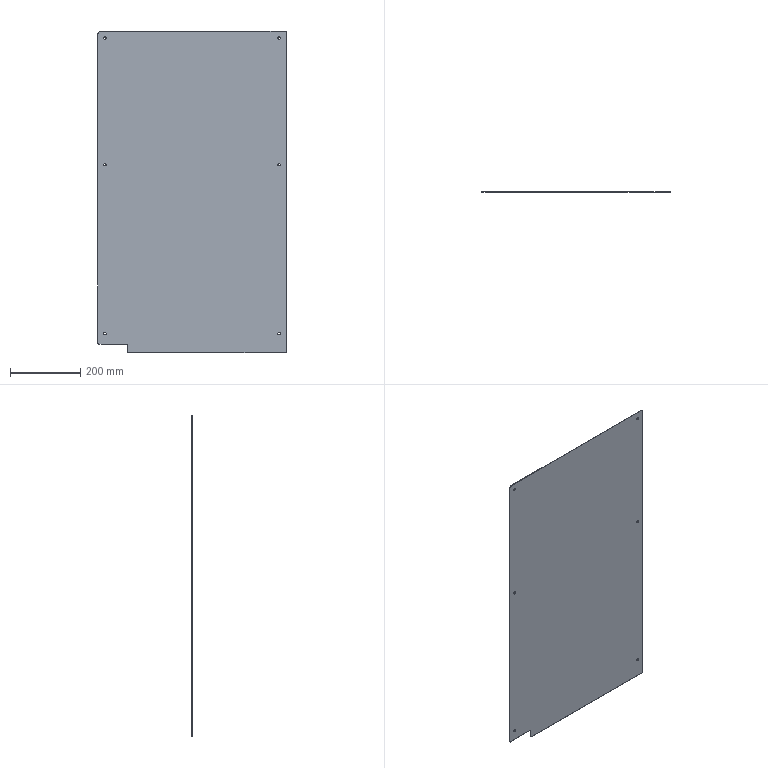Part | SolidWorks | features Fillet 4, ICE 4, FlatPattern 1, HoleWzd 1, SMBaseFlange 1, SheetMetal 1 | 1 solid | 26 faces | box 535 x 1.2 x 915 mm | volume 584570 mm3 | cylinder 18 | plane 8 | commonest cylinder face diameters 7 x12 6 x5 20 x1
STEP:
#1=CARTESIAN_POINT('',(20.,-1.2,-863.5));
#2=VERTEX_POINT('',#1);
#3=CARTESIAN_POINT('',(20.,-1.2,-856.5));
#4=VERTEX_POINT('',#3);
#5=CARTESIAN_POINT('',(20.,-1.2,-860.));
#6=DIRECTION('',(0.,1.,0.));
#7=DIRECTION('',(0.,0.,1.));
#8=AXIS2_PLACEMENT_3D('',#5,#6,#7);
#9=CIRCLE('',#8,3.5);
#10=EDGE_CURVE('',#2,#4,#9,.T.);
#11=ORIENTED_EDGE('',*,*,#10,.F.);
#12=CARTESIAN_POINT('',(20.,0.,-863.5));
#13=VERTEX_POINT('',#12);
#14=CARTESIAN_POINT('',(20.,0.,-863.5));
#15=DIRECTION('',(0.,1.,0.));
#16=VECTOR('',#15,1000.);
#17=LINE('',#14,#16);
#18=EDGE_CURVE('',#2,#13,#17,.T.);
#19=ORIENTED_EDGE('',*,*,#18,.T.);
#20=CARTESIAN_POINT('',(20.,0.,-856.5));
#21=VERTEX_POINT('',#20);
#22=CARTESIAN_POINT('',(20.,0.,-860.));
#23=DIRECTION('',(0.,1.,0.));
#24=DIRECTION('',(0.,0.,1.));
#25=AXIS2_PLACEMENT_3D('',#22,#23,#24);
#26=CIRCLE('',#25,3.5);
#27=EDGE_CURVE('',#13,#21,#26,.T.);
#28=ORIENTED_EDGE('',*,*,#27,.T.);
#29=CARTESIAN_POINT('',(20.,0.,-856.5));
#30=DIRECTION('',(0.,1.,0.));
#31=VECTOR('',#30,1000.);
#32=LINE('',#29,#31);
#33=EDGE_CURVE('',#4,#21,#32,.T.);
#34=ORIENTED_EDGE('',*,*,#33,.F.);
#35=EDGE_LOOP('',(#11,#19,#28,#34));
#36=FACE_OUTER_BOUND('',#35,.T.);
#37=CARTESIAN_POINT('',(20.,0.,-860.));
#38=DIRECTION('',(0.,1.,0.));
#39=DIRECTION('',(0.,0.,1.));
#40=AXIS2_PLACEMENT_3D('',#37,#38,#39);
#41=CYLINDRICAL_SURFACE('',#40,3.5);
#42=ADVANCED_FACE('',(#36),#41,.F.);
#43=CARTESIAN_POINT('',(20.,-1.2,-23.5));
#44=VERTEX_POINT('',#43);
#45=CARTESIAN_POINT('',(20.,-1.2,-16.5));
#46=VERTEX_POINT('',#45);
#47=CARTESIAN_POINT('',(20.,-1.2,-20.));
#48=DIRECTION('',(0.,1.,0.));
#49=DIRECTION('',(0.,0.,1.));
#50=AXIS2_PLACEMENT_3D('',#47,#48,#49);
#51=CIRCLE('',#50,3.5);
#52=EDGE_CURVE('',#44,#46,#51,.T.);
#53=ORIENTED_EDGE('',*,*,#52,.F.);
#54=CARTESIAN_POINT('',(20.,0.,-23.5));
#55=VERTEX_POINT('',#54);
#56=CARTESIAN_POINT('',(20.,0.,-23.5));
#57=DIRECTION('',(0.,1.,0.));
#58=VECTOR('',#57,1000.);
#59=LINE('',#56,#58);
#60=EDGE_CURVE('',#44,#55,#59,.T.);
#61=ORIENTED_EDGE('',*,*,#60,.T.);
#62=CARTESIAN_POINT('',(20.,0.,-16.5));
#63=VERTEX_POINT('',#62);
#64=CARTESIAN_POINT('',(20.,0.,-20.));
#65=DIRECTION('',(0.,1.,0.));
#66=DIRECTION('',(0.,0.,1.));
#67=AXIS2_PLACEMENT_3D('',#64,#65,#66);
#68=CIRCLE('',#67,3.5);
#69=EDGE_CURVE('',#55,#63,#68,.T.);
#70=ORIENTED_EDGE('',*,*,#69,.T.);
#71=CARTESIAN_POINT('',(20.,0.,-16.5));
#72=DIRECTION('',(0.,1.,0.));
#73=VECTOR('',#72,1000.);
#74=LINE('',#71,#73);
#75=EDGE_CURVE('',#46,#63,#74,.T.);
#76=ORIENTED_EDGE('',*,*,#75,.F.);
#77=EDGE_LOOP('',(#53,#61,#70,#76));
#78=FACE_OUTER_BOUND('',#77,.T.);
#79=CARTESIAN_POINT('',(20.,0.,-20.));
#80=DIRECTION('',(0.,1.,0.));
#81=DIRECTION('',(0.,0.,1.));
#82=AXIS2_PLACEMENT_3D('',#79,#80,#81);
#83=CYLINDRICAL_SURFACE('',#82,3.5);
#84=ADVANCED_FACE('',(#78),#83,.F.);
#85=CARTESIAN_POINT('',(515.,-1.2,-23.5));
#86=VERTEX_POINT('',#85);
#87=CARTESIAN_POINT('',(515.,-1.2,-16.5));
#88=VERTEX_POINT('',#87);
#89=CARTESIAN_POINT('',(515.,-1.2,-20.));
#90=DIRECTION('',(0.,1.,0.));
#91=DIRECTION('',(0.,0.,1.));
#92=AXIS2_PLACEMENT_3D('',#89,#90,#91);
#93=CIRCLE('',#92,3.5);
#94=EDGE_CURVE('',#86,#88,#93,.T.);
#95=ORIENTED_EDGE('',*,*,#94,.F.);
#96=CARTESIAN_POINT('',(515.,0.,-23.5));
#97=VERTEX_POINT('',#96);
#98=CARTESIAN_POINT('',(515.,0.,-23.5));
#99=DIRECTION('',(0.,1.,0.));
#100=VECTOR('',#99,1000.);
#101=LINE('',#98,#100);
#102=EDGE_CURVE('',#86,#97,#101,.T.);
#103=ORIENTED_EDGE('',*,*,#102,.T.);
#104=CARTESIAN_POINT('',(515.,0.,-16.5));
#105=VERTEX_POINT('',#104);
#106=CARTESIAN_POINT('',(515.,0.,-20.));
#107=DIRECTION('',(0.,1.,0.));
#108=DIRECTION('',(0.,0.,1.));
#109=AXIS2_PLACEMENT_3D('',#106,#107,#108);
#110=CIRCLE('',#109,3.5);
#111=EDGE_CURVE('',#97,#105,#110,.T.);
#112=ORIENTED_EDGE('',*,*,#111,.T.);
#113=CARTESIAN_POINT('',(515.,0.,-16.5));
#114=DIRECTION('',(0.,1.,0.));
#115=VECTOR('',#114,1000.);
#116=LINE('',#113,#115);
#117=EDGE_CURVE('',#88,#105,#116,.T.);
#118=ORIENTED_EDGE('',*,*,#117,.F.);
#119=EDGE_LOOP('',(#95,#103,#112,#118));
#120=FACE_OUTER_BOUND('',#119,.T.);
#121=CARTESIAN_POINT('',(515.,0.,-20.));
#122=DIRECTION('',(0.,1.,0.));
#123=DIRECTION('',(0.,0.,1.));
#124=AXIS2_PLACEMENT_3D('',#121,#122,#123);
#125=CYLINDRICAL_SURFACE('',#124,3.5);
#126=ADVANCED_FACE('',(#120),#125,.F.);
#127=CARTESIAN_POINT('',(20.,-1.2,-383.5));
#128=VERTEX_POINT('',#127);
#129=CARTESIAN_POINT('',(20.,-1.2,-376.5));
#130=VERTEX_POINT('',#129);
#131=CARTESIAN_POINT('',(20.,-1.2,-380.));
#132=DIRECTION('',(0.,1.,0.));
#133=DIRECTION('',(0.,0.,1.));
#134=AXIS2_PLACEMENT_3D('',#131,#132,#133);
#135=CIRCLE('',#134,3.5);
#136=EDGE_CURVE('',#128,#130,#135,.T.);
#137=ORIENTED_EDGE('',*,*,#136,.F.);
#138=CARTESIAN_POINT('',(20.,0.,-383.5));
#139=VERTEX_POINT('',#138);
#140=CARTESIAN_POINT('',(20.,0.,-383.5));
#141=DIRECTION('',(0.,1.,0.));
#142=VECTOR('',#141,1000.);
#143=LINE('',#140,#142);
#144=EDGE_CURVE('',#128,#139,#143,.T.);
#145=ORIENTED_EDGE('',*,*,#144,.T.);
#146=CARTESIAN_POINT('',(20.,0.,-376.5));
#147=VERTEX_POINT('',#146);
#148=CARTESIAN_POINT('',(20.,0.,-380.));
#149=DIRECTION('',(0.,1.,0.));
#150=DIRECTION('',(0.,0.,1.));
#151=AXIS2_PLACEMENT_3D('',#148,#149,#150);
#152=CIRCLE('',#151,3.5);
#153=EDGE_CURVE('',#139,#147,#152,.T.);
#154=ORIENTED_EDGE('',*,*,#153,.T.);
#155=CARTESIAN_POINT('',(20.,0.,-376.5));
#156=DIRECTION('',(0.,1.,0.));
#157=VECTOR('',#156,1000.);
#158=LINE('',#155,#157);
#159=EDGE_CURVE('',#130,#147,#158,.T.);
#160=ORIENTED_EDGE('',*,*,#159,.F.);
#161=EDGE_LOOP('',(#137,#145,#154,#160));
#162=FACE_OUTER_BOUND('',#161,.T.);
#163=CARTESIAN_POINT('',(20.,0.,-380.));
#164=DIRECTION('',(0.,1.,0.));
#165=DIRECTION('',(0.,0.,1.));
#166=AXIS2_PLACEMENT_3D('',#163,#164,#165);
#167=CYLINDRICAL_SURFACE('',#166,3.5);
#168=ADVANCED_FACE('',(#162),#167,.F.);
#169=CARTESIAN_POINT('',(515.,-1.2,-383.5));
#170=VERTEX_POINT('',#169);
#171=CARTESIAN_POINT('',(515.,-1.2,-376.5));
#172=VERTEX_POINT('',#171);
#173=CARTESIAN_POINT('',(515.,-1.2,-380.));
#174=DIRECTION('',(0.,1.,0.));
#175=DIRECTION('',(0.,0.,1.));
#176=AXIS2_PLACEMENT_3D('',#173,#174,#175);
#177=CIRCLE('',#176,3.5);
#178=EDGE_CURVE('',#170,#172,#177,.T.);
#179=ORIENTED_EDGE('',*,*,#178,.F.);
#180=CARTESIAN_POINT('',(515.,0.,-383.5));
#181=VERTEX_POINT('',#180);
#182=CARTESIAN_POINT('',(515.,0.,-383.5));
#183=DIRECTION('',(0.,1.,0.));
#184=VECTOR('',#183,1000.);
#185=LINE('',#182,#184);
#186=EDGE_CURVE('',#170,#181,#185,.T.);
#187=ORIENTED_EDGE('',*,*,#186,.T.);
#188=CARTESIAN_POINT('',(515.,0.,-376.5));
#189=VERTEX_POINT('',#188);
#190=CARTESIAN_POINT('',(515.,0.,-380.));
#191=DIRECTION('',(0.,1.,0.));
#192=DIRECTION('',(0.,0.,1.));
#193=AXIS2_PLACEMENT_3D('',#190,#191,#192);
#194=CIRCLE('',#193,3.5);
#195=EDGE_CURVE('',#181,#189,#194,.T.);
#196=ORIENTED_EDGE('',*,*,#195,.T.);
#197=CARTESIAN_POINT('',(515.,0.,-376.5));
#198=DIRECTION('',(0.,1.,0.));
#199=VECTOR('',#198,1000.);
#200=LINE('',#197,#199);
#201=EDGE_CURVE('',#172,#189,#200,.T.);
#202=ORIENTED_EDGE('',*,*,#201,.F.);
#203=EDGE_LOOP('',(#179,#187,#196,#202));
#204=FACE_OUTER_BOUND('',#203,.T.);
#205=CARTESIAN_POINT('',(515.,0.,-380.));
#206=DIRECTION('',(0.,1.,0.));
#207=DIRECTION('',(0.,0.,1.));
#208=AXIS2_PLACEMENT_3D('',#205,#206,#207);
#209=CYLINDRICAL_SURFACE('',#208,3.5);
#210=ADVANCED_FACE('',(#204),#209,.F.);
#211=CARTESIAN_POINT('',(515.,-1.2,-863.5));
#212=VERTEX_POINT('',#211);
#213=CARTESIAN_POINT('',(515.,-1.2,-856.5));
#214=VERTEX_POINT('',#213);
#215=CARTESIAN_POINT('',(515.,-1.2,-860.));
#216=DIRECTION('',(0.,1.,0.));
#217=DIRECTION('',(0.,0.,1.));
#218=AXIS2_PLACEMENT_3D('',#215,#216,#217);
#219=CIRCLE('',#218,3.5);
#220=EDGE_CURVE('',#212,#214,#219,.T.);
#221=ORIENTED_EDGE('',*,*,#220,.F.);
#222=CARTESIAN_POINT('',(515.,0.,-863.5));
#223=VERTEX_POINT('',#222);
#224=CARTESIAN_POINT('',(515.,0.,-863.5));
#225=DIRECTION('',(0.,1.,0.));
#226=VECTOR('',#225,1000.);
#227=LINE('',#224,#226);
#228=EDGE_CURVE('',#212,#223,#227,.T.);
#229=ORIENTED_EDGE('',*,*,#228,.T.);
#230=CARTESIAN_POINT('',(515.,0.,-856.5));
#231=VERTEX_POINT('',#230);
#232=CARTESIAN_POINT('',(515.,0.,-860.));
#233=DIRECTION('',(0.,1.,0.));
#234=DIRECTION('',(0.,0.,1.));
#235=AXIS2_PLACEMENT_3D('',#232,#233,#234);
#236=CIRCLE('',#235,3.5);
#237=EDGE_CURVE('',#223,#231,#236,.T.);
#238=ORIENTED_EDGE('',*,*,#237,.T.);
#239=CARTESIAN_POINT('',(515.,0.,-856.5));
#240=DIRECTION('',(0.,1.,0.));
#241=VECTOR('',#240,1000.);
#242=LINE('',#239,#241);
#243=EDGE_CURVE('',#214,#231,#242,.T.);
#244=ORIENTED_EDGE('',*,*,#243,.F.);
#245=EDGE_LOOP('',(#221,#229,#238,#244));
#246=FACE_OUTER_BOUND('',#245,.T.);
#247=CARTESIAN_POINT('',(515.,0.,-860.));
#248=DIRECTION('',(0.,1.,0.));
#249=DIRECTION('',(0.,0.,1.));
#250=AXIS2_PLACEMENT_3D('',#247,#248,#249);
#251=CYLINDRICAL_SURFACE('',#250,3.5);
#252=ADVANCED_FACE('',(#246),#251,.F.);
#253=CARTESIAN_POINT('',(20.,0.,-860.));
#254=DIRECTION('',(0.,1.,0.));
#255=DIRECTION('',(0.,0.,1.));
#256=AXIS2_PLACEMENT_3D('',#253,#254,#255);
#257=CIRCLE('',#256,3.5);
#258=EDGE_CURVE('',#21,#13,#257,.T.);
#259=ORIENTED_EDGE('',*,*,#258,.F.);
#260=ORIENTED_EDGE('',*,*,#27,.F.);
#261=EDGE_LOOP('',(#259,#260));
#262=FACE_BOUND('',#261,.T.);
#263=CARTESIAN_POINT('',(20.,0.,-20.));
#264=DIRECTION('',(0.,1.,0.));
#265=DIRECTION('',(0.,0.,1.));
#266=AXIS2_PLACEMENT_3D('',#263,#264,#265);
#267=CIRCLE('',#266,3.5);
#268=EDGE_CURVE('',#63,#55,#267,.T.);
#269=ORIENTED_EDGE('',*,*,#268,.F.);
#270=ORIENTED_EDGE('',*,*,#69,.F.);
#271=EDGE_LOOP('',(#269,#270));
#272=FACE_BOUND('',#271,.T.);
#273=CARTESIAN_POINT('',(515.,0.,-20.));
#274=DIRECTION('',(0.,1.,0.));
#275=DIRECTION('',(0.,0.,1.));
#276=AXIS2_PLACEMENT_3D('',#273,#274,#275);
#277=CIRCLE('',#276,3.5);
#278=EDGE_CURVE('',#105,#97,#277,.T.);
#279=ORIENTED_EDGE('',*,*,#278,.F.);
#280=ORIENTED_EDGE('',*,*,#111,.F.);
#281=EDGE_LOOP('',(#279,#280));
#282=FACE_BOUND('',#281,.T.);
#283=CARTESIAN_POINT('',(515.,0.,-380.));
#284=DIRECTION('',(0.,1.,0.));
#285=DIRECTION('',(0.,0.,1.));
#286=AXIS2_PLACEMENT_3D('',#283,#284,#285);
#287=CIRCLE('',#286,3.5);
#288=EDGE_CURVE('',#189,#181,#287,.T.);
#289=ORIENTED_EDGE('',*,*,#288,.F.);
#290=ORIENTED_EDGE('',*,*,#195,.F.);
#291=EDGE_LOOP('',(#289,#290));
#292=FACE_BOUND('',#291,.T.);
#293=CARTESIAN_POINT('',(515.,0.,-860.));
#294=DIRECTION('',(0.,1.,0.));
#295=DIRECTION('',(0.,0.,1.));
#296=AXIS2_PLACEMENT_3D('',#293,#294,#295);
#297=CIRCLE('',#296,3.5);
#298=EDGE_CURVE('',#231,#223,#297,.T.);
#299=ORIENTED_EDGE('',*,*,#298,.F.);
#300=ORIENTED_EDGE('',*,*,#237,.F.);
#301=EDGE_LOOP('',(#299,#300));
#302=FACE_BOUND('',#301,.T.);
#303=CARTESIAN_POINT('',(535.,0.,-912.));
#304=VERTEX_POINT('',#303);
#305=CARTESIAN_POINT('',(535.,0.,-3.));
#306=VERTEX_POINT('',#305);
#307=CARTESIAN_POINT('',(535.,0.,-915.));
#308=DIRECTION('',(0.,0.,1.));
#309=VECTOR('',#308,1000.);
#310=LINE('',#307,#309);
#311=EDGE_CURVE('',#304,#306,#310,.T.);
#312=ORIENTED_EDGE('',*,*,#311,.F.);
#313=CARTESIAN_POINT('',(532.,0.,-915.));
#314=VERTEX_POINT('',#313);
#315=CARTESIAN_POINT('',(532.,0.,-912.));
#316=DIRECTION('',(0.,1.,0.));
#317=DIRECTION('',(0.,0.,-1.));
#318=AXIS2_PLACEMENT_3D('',#315,#316,#317);
#319=CIRCLE('',#318,3.);
#320=EDGE_CURVE('',#304,#314,#319,.T.);
#321=ORIENTED_EDGE('',*,*,#320,.T.);
#322=CARTESIAN_POINT('',(88.,0.,-915.));
#323=VERTEX_POINT('',#322);
#324=CARTESIAN_POINT('',(0.,0.,-915.));
#325=DIRECTION('',(-1.,0.,0.));
#326=VECTOR('',#325,1000.);
#327=LINE('',#324,#326);
#328=EDGE_CURVE('',#314,#323,#327,.T.);
#329=ORIENTED_EDGE('',*,*,#328,.T.);
#330=CARTESIAN_POINT('',(85.,0.,-912.));
#331=VERTEX_POINT('',#330);
#332=CARTESIAN_POINT('',(88.,0.,-912.));
#333=DIRECTION('',(0.,1.,0.));
#334=DIRECTION('',(0.,0.,-1.));
#335=AXIS2_PLACEMENT_3D('',#332,#333,#334);
#336=CIRCLE('',#335,3.);
#337=EDGE_CURVE('',#323,#331,#336,.T.);
#338=ORIENTED_EDGE('',*,*,#337,.T.);
#339=CARTESIAN_POINT('',(85.,0.,-893.));
#340=VERTEX_POINT('',#339);
#341=CARTESIAN_POINT('',(85.,0.,-915.));
#342=DIRECTION('',(0.,0.,-1.));
#343=VECTOR('',#342,1000.);
#344=LINE('',#341,#343);
#345=EDGE_CURVE('',#340,#331,#344,.T.);
#346=ORIENTED_EDGE('',*,*,#345,.F.);
#347=CARTESIAN_POINT('',(82.,0.,-890.));
#348=VERTEX_POINT('',#347);
#349=CARTESIAN_POINT('',(82.,0.,-893.));
#350=DIRECTION('',(0.,-1.,0.));
#351=DIRECTION('',(0.,0.,-1.));
#352=AXIS2_PLACEMENT_3D('',#349,#350,#351);
#353=CIRCLE('',#352,3.);
#354=EDGE_CURVE('',#340,#348,#353,.T.);
#355=ORIENTED_EDGE('',*,*,#354,.T.);
#356=CARTESIAN_POINT('',(3.,0.,-890.));
#357=VERTEX_POINT('',#356);
#358=CARTESIAN_POINT('',(0.,0.,-890.));
#359=DIRECTION('',(1.,0.,0.));
#360=VECTOR('',#359,1000.);
#361=LINE('',#358,#360);
#362=EDGE_CURVE('',#357,#348,#361,.T.);
#363=ORIENTED_EDGE('',*,*,#362,.F.);
#364=CARTESIAN_POINT('',(0.,0.,-887.));
#365=VERTEX_POINT('',#364);
#366=CARTESIAN_POINT('',(3.,0.,-887.));
#367=DIRECTION('',(0.,1.,0.));
#368=DIRECTION('',(0.,0.,-1.));
#369=AXIS2_PLACEMENT_3D('',#366,#367,#368);
#370=CIRCLE('',#369,3.);
#371=EDGE_CURVE('',#357,#365,#370,.T.);
#372=ORIENTED_EDGE('',*,*,#371,.T.);
#373=CARTESIAN_POINT('',(0.,0.,-10.));
#374=VERTEX_POINT('',#373);
#375=CARTESIAN_POINT('',(0.,0.,0.));
#376=DIRECTION('',(0.,0.,1.));
#377=VECTOR('',#376,1000.);
#378=LINE('',#375,#377);
#379=EDGE_CURVE('',#365,#374,#378,.T.);
#380=ORIENTED_EDGE('',*,*,#379,.T.);
#381=CARTESIAN_POINT('',(10.,0.,0.));
#382=VERTEX_POINT('',#381);
#383=CARTESIAN_POINT('',(10.,0.,-10.));
#384=DIRECTION('',(0.,1.,0.));
#385=DIRECTION('',(0.,0.,-1.));
#386=AXIS2_PLACEMENT_3D('',#383,#384,#385);
#387=CIRCLE('',#386,10.);
#388=EDGE_CURVE('',#374,#382,#387,.T.);
#389=ORIENTED_EDGE('',*,*,#388,.T.);
#390=CARTESIAN_POINT('',(532.,0.,0.));
#391=VERTEX_POINT('',#390);
#392=CARTESIAN_POINT('',(0.,0.,0.));
#393=DIRECTION('',(1.,0.,0.));
#394=VECTOR('',#393,1000.);
#395=LINE('',#392,#394);
#396=EDGE_CURVE('',#382,#391,#395,.T.);
#397=ORIENTED_EDGE('',*,*,#396,.T.);
#398=CARTESIAN_POINT('',(532.,0.,-3.));
#399=DIRECTION('',(0.,1.,0.));
#400=DIRECTION('',(0.,0.,-1.));
#401=AXIS2_PLACEMENT_3D('',#398,#399,#400);
#402=CIRCLE('',#401,3.);
#403=EDGE_CURVE('',#391,#306,#402,.T.);
#404=ORIENTED_EDGE('',*,*,#403,.T.);
#405=EDGE_LOOP('',(#312,#321,#329,#338,#346,#355,#363,#372,#380,#389,#397,#404));
#406=FACE_OUTER_BOUND('',#405,.T.);
#407=CARTESIAN_POINT('',(20.,0.,-380.));
#408=DIRECTION('',(0.,1.,0.));
#409=DIRECTION('',(0.,0.,1.));
#410=AXIS2_PLACEMENT_3D('',#407,#408,#409);
#411=CIRCLE('',#410,3.5);
#412=EDGE_CURVE('',#147,#139,#411,.T.);
#413=ORIENTED_EDGE('',*,*,#412,.F.);
#414=ORIENTED_EDGE('',*,*,#153,.F.);
#415=EDGE_LOOP('',(#413,#414));
#416=FACE_BOUND('',#415,.T.);
#417=CARTESIAN_POINT('',(0.,0.,0.));
#418=DIRECTION('',(0.,-1.,0.));
#419=DIRECTION('',(0.,0.,-1.));
#420=AXIS2_PLACEMENT_3D('',#417,#418,#419);
#421=PLANE('',#420);
#422=ADVANCED_FACE('',(#262,#272,#282,#292,#302,#406,#416),#421,.F.);
#423=ORIENTED_EDGE('',*,*,#328,.F.);
#424=CARTESIAN_POINT('',(532.,-1.2,-915.));
#425=VERTEX_POINT('',#424);
#426=CARTESIAN_POINT('',(532.,-1.2,-915.));
#427=DIRECTION('',(0.,-1.,0.));
#428=VECTOR('',#427,1000.);
#429=LINE('',#426,#428);
#430=EDGE_CURVE('',#314,#425,#429,.T.);
#431=ORIENTED_EDGE('',*,*,#430,.T.);
#432=CARTESIAN_POINT('',(88.,-1.2,-915.));
#433=VERTEX_POINT('',#432);
#434=CARTESIAN_POINT('',(0.,-1.2,-915.));
#435=DIRECTION('',(-1.,0.,0.));
#436=VECTOR('',#435,1000.);
#437=LINE('',#434,#436);
#438=EDGE_CURVE('',#425,#433,#437,.T.);
#439=ORIENTED_EDGE('',*,*,#438,.T.);
#440=CARTESIAN_POINT('',(88.,0.,-915.));
#441=DIRECTION('',(0.,1.,0.));
#442=VECTOR('',#441,1000.);
#443=LINE('',#440,#442);
#444=EDGE_CURVE('',#433,#323,#443,.T.);
#445=ORIENTED_EDGE('',*,*,#444,.T.);
#446=EDGE_LOOP('',(#423,#431,#439,#445));
#447=FACE_OUTER_BOUND('',#446,.T.);
#448=CARTESIAN_POINT('',(0.,-1.2,-915.));
#449=DIRECTION('',(0.,0.,-1.));
#450=DIRECTION('',(-1.,0.,0.));
#451=AXIS2_PLACEMENT_3D('',#448,#449,#450);
#452=PLANE('',#451);
#453=ADVANCED_FACE('',(#447),#452,.T.);
#454=CARTESIAN_POINT('',(10.,-1.2,0.));
#455=VERTEX_POINT('',#454);
#456=CARTESIAN_POINT('',(532.,-1.2,0.));
#457=VERTEX_POINT('',#456);
#458=CARTESIAN_POINT('',(0.,-1.2,0.));
#459=DIRECTION('',(1.,0.,0.));
#460=VECTOR('',#459,1000.);
#461=LINE('',#458,#460);
#462=EDGE_CURVE('',#455,#457,#461,.T.);
#463=ORIENTED_EDGE('',*,*,#462,.T.);
#464=CARTESIAN_POINT('',(532.,0.,0.));
#465=DIRECTION('',(0.,1.,0.));
#466=VECTOR('',#465,1000.);
#467=LINE('',#464,#466);
#468=EDGE_CURVE('',#457,#391,#467,.T.);
#469=ORIENTED_EDGE('',*,*,#468,.T.);
#470=ORIENTED_EDGE('',*,*,#396,.F.);
#471=CARTESIAN_POINT('',(10.,-1.2,0.));
#472=DIRECTION('',(0.,-1.,0.));
#473=VECTOR('',#472,1000.);
#474=LINE('',#471,#473);
#475=EDGE_CURVE('',#382,#455,#474,.T.);
#476=ORIENTED_EDGE('',*,*,#475,.T.);
#477=EDGE_LOOP('',(#463,#469,#470,#476));
#478=FACE_OUTER_BOUND('',#477,.T.);
#479=CARTESIAN_POINT('',(0.,-1.2,0.));
#480=DIRECTION('',(0.,0.,1.));
#481=DIRECTION('',(1.,0.,0.));
#482=AXIS2_PLACEMENT_3D('',#479,#480,#481);
#483=PLANE('',#482);
#484=ADVANCED_FACE('',(#478),#483,.T.);
#485=CARTESIAN_POINT('',(20.,-1.2,-860.));
#486=DIRECTION('',(0.,1.,0.));
#487=DIRECTION('',(0.,0.,1.));
#488=AXIS2_PLACEMENT_3D('',#485,#486,#487);
#489=CIRCLE('',#488,3.5);
#490=EDGE_CURVE('',#4,#2,#489,.T.);
#491=ORIENTED_EDGE('',*,*,#490,.T.);
#492=ORIENTED_EDGE('',*,*,#10,.T.);
#493=EDGE_LOOP('',(#491,#492));
#494=FACE_BOUND('',#493,.T.);
#495=CARTESIAN_POINT('',(20.,-1.2,-20.));
#496=DIRECTION('',(0.,1.,0.));
#497=DIRECTION('',(0.,0.,1.));
#498=AXIS2_PLACEMENT_3D('',#495,#496,#497);
#499=CIRCLE('',#498,3.5);
#500=EDGE_CURVE('',#46,#44,#499,.T.);
#501=ORIENTED_EDGE('',*,*,#500,.T.);
#502=ORIENTED_EDGE('',*,*,#52,.T.);
#503=EDGE_LOOP('',(#501,#502));
#504=FACE_BOUND('',#503,.T.);
#505=CARTESIAN_POINT('',(515.,-1.2,-20.));
#506=DIRECTION('',(0.,1.,0.));
#507=DIRECTION('',(0.,0.,1.));
#508=AXIS2_PLACEMENT_3D('',#505,#506,#507);
#509=CIRCLE('',#508,3.5);
#510=EDGE_CURVE('',#88,#86,#509,.T.);
#511=ORIENTED_EDGE('',*,*,#510,.T.);
#512=ORIENTED_EDGE('',*,*,#94,.T.);
#513=EDGE_LOOP('',(#511,#512));
#514=FACE_BOUND('',#513,.T.);
#515=CARTESIAN_POINT('',(20.,-1.2,-380.));
#516=DIRECTION('',(0.,1.,0.));
#517=DIRECTION('',(0.,0.,1.));
#518=AXIS2_PLACEMENT_3D('',#515,#516,#517);
#519=CIRCLE('',#518,3.5);
#520=EDGE_CURVE('',#130,#128,#519,.T.);
#521=ORIENTED_EDGE('',*,*,#520,.T.);
#522=ORIENTED_EDGE('',*,*,#136,.T.);
#523=EDGE_LOOP('',(#521,#522));
#524=FACE_BOUND('',#523,.T.);
#525=CARTESIAN_POINT('',(515.,-1.2,-380.));
#526=DIRECTION('',(0.,1.,0.));
#527=DIRECTION('',(0.,0.,1.));
#528=AXIS2_PLACEMENT_3D('',#525,#526,#527);
#529=CIRCLE('',#528,3.5);
#530=EDGE_CURVE('',#172,#170,#529,.T.);
#531=ORIENTED_EDGE('',*,*,#530,.T.);
#532=ORIENTED_EDGE('',*,*,#178,.T.);
#533=EDGE_LOOP('',(#531,#532));
#534=FACE_BOUND('',#533,.T.);
#535=CARTESIAN_POINT('',(515.,-1.2,-860.));
#536=DIRECTION('',(0.,1.,0.));
#537=DIRECTION('',(0.,0.,1.));
#538=AXIS2_PLACEMENT_3D('',#535,#536,#537);
#539=CIRCLE('',#538,3.5);
#540=EDGE_CURVE('',#214,#212,#539,.T.);
#541=ORIENTED_EDGE('',*,*,#540,.T.);
#542=ORIENTED_EDGE('',*,*,#220,.T.);
#543=EDGE_LOOP('',(#541,#542));
#544=FACE_BOUND('',#543,.T.);
#545=ORIENTED_EDGE('',*,*,#438,.F.);
#546=CARTESIAN_POINT('',(535.,-1.2,-912.));
#547=VERTEX_POINT('',#546);
#548=CARTESIAN_POINT('',(532.,-1.2,-912.));
#549=DIRECTION('',(0.,-1.,0.));
#550=DIRECTION('',(0.,0.,-1.));
#551=AXIS2_PLACEMENT_3D('',#548,#549,#550);
#552=CIRCLE('',#551,3.);
#553=EDGE_CURVE('',#425,#547,#552,.T.);
#554=ORIENTED_EDGE('',*,*,#553,.T.);
#555=CARTESIAN_POINT('',(535.,-1.2,-3.));
#556=VERTEX_POINT('',#555);
#557=CARTESIAN_POINT('',(535.,-1.2,0.));
#558=DIRECTION('',(0.,0.,-1.));
#559=VECTOR('',#558,1000.);
#560=LINE('',#557,#559);
#561=EDGE_CURVE('',#556,#547,#560,.T.);
#562=ORIENTED_EDGE('',*,*,#561,.F.);
#563=CARTESIAN_POINT('',(532.,-1.2,-3.));
#564=DIRECTION('',(0.,-1.,0.));
#565=DIRECTION('',(0.,0.,-1.));
#566=AXIS2_PLACEMENT_3D('',#563,#564,#565);
#567=CIRCLE('',#566,3.);
#568=EDGE_CURVE('',#556,#457,#567,.T.);
#569=ORIENTED_EDGE('',*,*,#568,.T.);
#570=ORIENTED_EDGE('',*,*,#462,.F.);
#571=CARTESIAN_POINT('',(0.,-1.2,-10.));
#572=VERTEX_POINT('',#571);
#573=CARTESIAN_POINT('',(10.,-1.2,-10.));
#574=DIRECTION('',(0.,-1.,0.));
#575=DIRECTION('',(0.,0.,-1.));
#576=AXIS2_PLACEMENT_3D('',#573,#574,#575);
#577=CIRCLE('',#576,10.);
#578=EDGE_CURVE('',#455,#572,#577,.T.);
#579=ORIENTED_EDGE('',*,*,#578,.T.);
#580=CARTESIAN_POINT('',(0.,-1.2,-887.));
#581=VERTEX_POINT('',#580);
#582=CARTESIAN_POINT('',(0.,-1.2,0.));
#583=DIRECTION('',(0.,0.,1.));
#584=VECTOR('',#583,1000.);
#585=LINE('',#582,#584);
#586=EDGE_CURVE('',#581,#572,#585,.T.);
#587=ORIENTED_EDGE('',*,*,#586,.F.);
#588=CARTESIAN_POINT('',(3.,-1.2,-890.));
#589=VERTEX_POINT('',#588);
#590=CARTESIAN_POINT('',(3.,-1.2,-887.));
#591=DIRECTION('',(0.,-1.,0.));
#592=DIRECTION('',(0.,0.,-1.));
#593=AXIS2_PLACEMENT_3D('',#590,#591,#592);
#594=CIRCLE('',#593,3.);
#595=EDGE_CURVE('',#581,#589,#594,.T.);
#596=ORIENTED_EDGE('',*,*,#595,.T.);
#597=CARTESIAN_POINT('',(82.,-1.2,-890.));
#598=VERTEX_POINT('',#597);
#599=CARTESIAN_POINT('',(0.,-1.2,-890.));
#600=DIRECTION('',(-1.,0.,0.));
#601=VECTOR('',#600,1000.);
#602=LINE('',#599,#601);
#603=EDGE_CURVE('',#598,#589,#602,.T.);
#604=ORIENTED_EDGE('',*,*,#603,.F.);
#605=CARTESIAN_POINT('',(85.,-1.2,-893.));
#606=VERTEX_POINT('',#605);
#607=CARTESIAN_POINT('',(82.,-1.2,-893.));
#608=DIRECTION('',(0.,1.,0.));
#609=DIRECTION('',(0.,0.,-1.));
#610=AXIS2_PLACEMENT_3D('',#607,#608,#609);
#611=CIRCLE('',#610,3.);
#612=EDGE_CURVE('',#598,#606,#611,.T.);
#613=ORIENTED_EDGE('',*,*,#612,.T.);
#614=CARTESIAN_POINT('',(85.,-1.2,-912.));
#615=VERTEX_POINT('',#614);
#616=CARTESIAN_POINT('',(85.,-1.2,0.));
#617=DIRECTION('',(0.,0.,1.));
#618=VECTOR('',#617,1000.);
#619=LINE('',#616,#618);
#620=EDGE_CURVE('',#615,#606,#619,.T.);
#621=ORIENTED_EDGE('',*,*,#620,.F.);
#622=CARTESIAN_POINT('',(88.,-1.2,-912.));
#623=DIRECTION('',(0.,-1.,0.));
#624=DIRECTION('',(0.,0.,-1.));
#625=AXIS2_PLACEMENT_3D('',#622,#623,#624);
#626=CIRCLE('',#625,3.);
#627=EDGE_CURVE('',#615,#433,#626,.T.);
#628=ORIENTED_EDGE('',*,*,#627,.T.);
#629=EDGE_LOOP('',(#545,#554,#562,#569,#570,#579,#587,#596,#604,#613,#621,#628));
#630=FACE_OUTER_BOUND('',#629,.T.);
#631=CARTESIAN_POINT('',(0.,-1.2,0.));
#632=DIRECTION('',(0.,-1.,0.));
#633=DIRECTION('',(0.,0.,-1.));
#634=AXIS2_PLACEMENT_3D('',#631,#632,#633);
#635=PLANE('',#634);
#636=ADVANCED_FACE('',(#494,#504,#514,#524,#534,#544,#630),#635,.T.);
#637=ORIENTED_EDGE('',*,*,#379,.F.);
#638=CARTESIAN_POINT('',(0.,-1.2,-887.));
#639=DIRECTION('',(0.,-1.,0.));
#640=VECTOR('',#639,1000.);
#641=LINE('',#638,#640);
#642=EDGE_CURVE('',#365,#581,#641,.T.);
#643=ORIENTED_EDGE('',*,*,#642,.T.);
#644=ORIENTED_EDGE('',*,*,#586,.T.);
#645=CARTESIAN_POINT('',(0.,-1.2,-10.));
#646=DIRECTION('',(0.,1.,0.));
#647=VECTOR('',#646,1000.);
#648=LINE('',#645,#647);
#649=EDGE_CURVE('',#572,#374,#648,.T.);
#650=ORIENTED_EDGE('',*,*,#649,.T.);
#651=EDGE_LOOP('',(#637,#643,#644,#650));
#652=FACE_OUTER_BOUND('',#651,.T.);
#653=CARTESIAN_POINT('',(0.,-1.2,0.));
#654=DIRECTION('',(-1.,0.,0.));
#655=DIRECTION('',(0.,0.,1.));
#656=AXIS2_PLACEMENT_3D('',#653,#654,#655);
#657=PLANE('',#656);
#658=ADVANCED_FACE('',(#652),#657,.T.);
#659=ORIENTED_EDGE('',*,*,#561,.T.);
#660=CARTESIAN_POINT('',(535.,0.,-912.));
#661=DIRECTION('',(0.,1.,0.));
#662=VECTOR('',#661,1000.);
#663=LINE('',#660,#662);
#664=EDGE_CURVE('',#547,#304,#663,.T.);
#665=ORIENTED_EDGE('',*,*,#664,.T.);
#666=ORIENTED_EDGE('',*,*,#311,.T.);
#667=CARTESIAN_POINT('',(535.,-1.2,-3.));
#668=DIRECTION('',(0.,-1.,0.));
#669=VECTOR('',#668,1000.);
#670=LINE('',#667,#669);
#671=EDGE_CURVE('',#306,#556,#670,.T.);
#672=ORIENTED_EDGE('',*,*,#671,.T.);
#673=EDGE_LOOP('',(#659,#665,#666,#672));
#674=FACE_OUTER_BOUND('',#673,.T.);
#675=CARTESIAN_POINT('',(535.,-10.,-915.));
#676=DIRECTION('',(-1.,0.,0.));
#677=DIRECTION('',(0.,0.,1.));
#678=AXIS2_PLACEMENT_3D('',#675,#676,#677);
#679=PLANE('',#678);
#680=ADVANCED_FACE('',(#674),#679,.F.);
#681=ORIENTED_EDGE('',*,*,#345,.T.);
#682=CARTESIAN_POINT('',(85.,-1.2,-912.));
#683=DIRECTION('',(0.,-1.,0.));
#684=VECTOR('',#683,1000.);
#685=LINE('',#682,#684);
#686=EDGE_CURVE('',#331,#615,#685,.T.);
#687=ORIENTED_EDGE('',*,*,#686,.T.);
#688=ORIENTED_EDGE('',*,*,#620,.T.);
#689=CARTESIAN_POINT('',(85.,0.,-893.));
#690=DIRECTION('',(0.,1.,0.));
#691=VECTOR('',#690,1000.);
#692=LINE('',#689,#691);
#693=EDGE_CURVE('',#606,#340,#692,.T.);
#694=ORIENTED_EDGE('',*,*,#693,.T.);
#695=EDGE_LOOP('',(#681,#687,#688,#694));
#696=FACE_OUTER_BOUND('',#695,.T.);
#697=CARTESIAN_POINT('',(85.,-10.,-915.));
#698=DIRECTION('',(1.,0.,0.));
#699=DIRECTION('',(0.,0.,-1.));
#700=AXIS2_PLACEMENT_3D('',#697,#698,#699);
#701=PLANE('',#700);
#702=ADVANCED_FACE('',(#696),#701,.F.);
#703=ORIENTED_EDGE('',*,*,#362,.T.);
#704=CARTESIAN_POINT('',(82.,-1.2,-890.));
#705=DIRECTION('',(0.,-1.,0.));
#706=VECTOR('',#705,1000.);
#707=LINE('',#704,#706);
#708=EDGE_CURVE('',#348,#598,#707,.T.);
#709=ORIENTED_EDGE('',*,*,#708,.T.);
#710=ORIENTED_EDGE('',*,*,#603,.T.);
#711=CARTESIAN_POINT('',(3.,0.,-890.));
#712=DIRECTION('',(0.,1.,0.));
#713=VECTOR('',#712,1000.);
#714=LINE('',#711,#713);
#715=EDGE_CURVE('',#589,#357,#714,.T.);
#716=ORIENTED_EDGE('',*,*,#715,.T.);
#717=EDGE_LOOP('',(#703,#709,#710,#716));
#718=FACE_OUTER_BOUND('',#717,.T.);
#719=CARTESIAN_POINT('',(0.,-10.,-890.));
#720=DIRECTION('',(0.,0.,1.));
#721=DIRECTION('',(1.,0.,0.));
#722=AXIS2_PLACEMENT_3D('',#719,#720,#721);
#723=PLANE('',#722);
#724=ADVANCED_FACE('',(#718),#723,.F.);
#725=ORIENTED_EDGE('',*,*,#578,.F.);
#726=ORIENTED_EDGE('',*,*,#475,.F.);
#727=ORIENTED_EDGE('',*,*,#388,.F.);
#728=ORIENTED_EDGE('',*,*,#649,.F.);
#729=EDGE_LOOP('',(#725,#726,#727,#728));
#730=FACE_OUTER_BOUND('',#729,.T.);
#731=CARTESIAN_POINT('',(10.,-1.2,-10.));
#732=DIRECTION('',(0.,1.,0.));
#733=DIRECTION('',(0.,0.,1.));
#734=AXIS2_PLACEMENT_3D('',#731,#732,#733);
#735=CYLINDRICAL_SURFACE('',#734,10.);
#736=ADVANCED_FACE('',(#730),#735,.T.);
#737=ORIENTED_EDGE('',*,*,#228,.F.);
#738=ORIENTED_EDGE('',*,*,#540,.F.);
#739=ORIENTED_EDGE('',*,*,#243,.T.);
#740=ORIENTED_EDGE('',*,*,#298,.T.);
#741=EDGE_LOOP('',(#737,#738,#739,#740));
#742=FACE_OUTER_BOUND('',#741,.T.);
#743=CARTESIAN_POINT('',(515.,0.,-860.));
#744=DIRECTION('',(0.,1.,0.));
#745=DIRECTION('',(0.,0.,1.));
#746=AXIS2_PLACEMENT_3D('',#743,#744,#745);
#747=CYLINDRICAL_SURFACE('',#746,3.5);
#748=ADVANCED_FACE('',(#742),#747,.F.);
#749=ORIENTED_EDGE('',*,*,#186,.F.);
#750=ORIENTED_EDGE('',*,*,#530,.F.);
#751=ORIENTED_EDGE('',*,*,#201,.T.);
#752=ORIENTED_EDGE('',*,*,#288,.T.);
#753=EDGE_LOOP('',(#749,#750,#751,#752));
#754=FACE_OUTER_BOUND('',#753,.T.);
#755=CARTESIAN_POINT('',(515.,0.,-380.));
#756=DIRECTION('',(0.,1.,0.));
#757=DIRECTION('',(0.,0.,1.));
#758=AXIS2_PLACEMENT_3D('',#755,#756,#757);
#759=CYLINDRICAL_SURFACE('',#758,3.5);
#760=ADVANCED_FACE('',(#754),#759,.F.);
#761=ORIENTED_EDGE('',*,*,#144,.F.);
#762=ORIENTED_EDGE('',*,*,#520,.F.);
#763=ORIENTED_EDGE('',*,*,#159,.T.);
#764=ORIENTED_EDGE('',*,*,#412,.T.);
#765=EDGE_LOOP('',(#761,#762,#763,#764));
#766=FACE_OUTER_BOUND('',#765,.T.);
#767=CARTESIAN_POINT('',(20.,0.,-380.));
#768=DIRECTION('',(0.,1.,0.));
#769=DIRECTION('',(0.,0.,1.));
#770=AXIS2_PLACEMENT_3D('',#767,#768,#769);
#771=CYLINDRICAL_SURFACE('',#770,3.5);
#772=ADVANCED_FACE('',(#766),#771,.F.);
#773=ORIENTED_EDGE('',*,*,#102,.F.);
#774=ORIENTED_EDGE('',*,*,#510,.F.);
#775=ORIENTED_EDGE('',*,*,#117,.T.);
#776=ORIENTED_EDGE('',*,*,#278,.T.);
#777=EDGE_LOOP('',(#773,#774,#775,#776));
#778=FACE_OUTER_BOUND('',#777,.T.);
#779=CARTESIAN_POINT('',(515.,0.,-20.));
#780=DIRECTION('',(0.,1.,0.));
#781=DIRECTION('',(0.,0.,1.));
#782=AXIS2_PLACEMENT_3D('',#779,#780,#781);
#783=CYLINDRICAL_SURFACE('',#782,3.5);
#784=ADVANCED_FACE('',(#778),#783,.F.);
#785=ORIENTED_EDGE('',*,*,#60,.F.);
#786=ORIENTED_EDGE('',*,*,#500,.F.);
#787=ORIENTED_EDGE('',*,*,#75,.T.);
#788=ORIENTED_EDGE('',*,*,#268,.T.);
#789=EDGE_LOOP('',(#785,#786,#787,#788));
#790=FACE_OUTER_BOUND('',#789,.T.);
#791=CARTESIAN_POINT('',(20.,0.,-20.));
#792=DIRECTION('',(0.,1.,0.));
#793=DIRECTION('',(0.,0.,1.));
#794=AXIS2_PLACEMENT_3D('',#791,#792,#793);
#795=CYLINDRICAL_SURFACE('',#794,3.5);
#796=ADVANCED_FACE('',(#790),#795,.F.);
#797=ORIENTED_EDGE('',*,*,#18,.F.);
#798=ORIENTED_EDGE('',*,*,#490,.F.);
#799=ORIENTED_EDGE('',*,*,#33,.T.);
#800=ORIENTED_EDGE('',*,*,#258,.T.);
#801=EDGE_LOOP('',(#797,#798,#799,#800));
#802=FACE_OUTER_BOUND('',#801,.T.);
#803=CARTESIAN_POINT('',(20.,0.,-860.));
#804=DIRECTION('',(0.,1.,0.));
#805=DIRECTION('',(0.,0.,1.));
#806=AXIS2_PLACEMENT_3D('',#803,#804,#805);
#807=CYLINDRICAL_SURFACE('',#806,3.5);
#808=ADVANCED_FACE('',(#802),#807,.F.);
#809=ORIENTED_EDGE('',*,*,#553,.F.);
#810=ORIENTED_EDGE('',*,*,#430,.F.);
#811=ORIENTED_EDGE('',*,*,#320,.F.);
#812=ORIENTED_EDGE('',*,*,#664,.F.);
#813=EDGE_LOOP('',(#809,#810,#811,#812));
#814=FACE_OUTER_BOUND('',#813,.T.);
#815=CARTESIAN_POINT('',(532.,-10.,-912.));
#816=DIRECTION('',(0.,-1.,0.));
#817=DIRECTION('',(0.,0.,-1.));
#818=AXIS2_PLACEMENT_3D('',#815,#816,#817);
#819=CYLINDRICAL_SURFACE('',#818,3.);
#820=ADVANCED_FACE('',(#814),#819,.T.);
#821=ORIENTED_EDGE('',*,*,#627,.F.);
#822=ORIENTED_EDGE('',*,*,#686,.F.);
#823=ORIENTED_EDGE('',*,*,#337,.F.);
#824=ORIENTED_EDGE('',*,*,#444,.F.);
#825=EDGE_LOOP('',(#821,#822,#823,#824));
#826=FACE_OUTER_BOUND('',#825,.T.);
#827=CARTESIAN_POINT('',(88.,-1.2,-912.));
#828=DIRECTION('',(0.,-1.,0.));
#829=DIRECTION('',(0.,0.,-1.));
#830=AXIS2_PLACEMENT_3D('',#827,#828,#829);
#831=CYLINDRICAL_SURFACE('',#830,3.);
#832=ADVANCED_FACE('',(#826),#831,.T.);
#833=ORIENTED_EDGE('',*,*,#612,.F.);
#834=ORIENTED_EDGE('',*,*,#708,.F.);
#835=ORIENTED_EDGE('',*,*,#354,.F.);
#836=ORIENTED_EDGE('',*,*,#693,.F.);
#837=EDGE_LOOP('',(#833,#834,#835,#836));
#838=FACE_OUTER_BOUND('',#837,.T.);
#839=CARTESIAN_POINT('',(82.,-10.,-893.));
#840=DIRECTION('',(0.,-1.,0.));
#841=DIRECTION('',(0.,0.,-1.));
#842=AXIS2_PLACEMENT_3D('',#839,#840,#841);
#843=CYLINDRICAL_SURFACE('',#842,3.);
#844=ADVANCED_FACE('',(#838),#843,.F.);
#845=ORIENTED_EDGE('',*,*,#595,.F.);
#846=ORIENTED_EDGE('',*,*,#642,.F.);
#847=ORIENTED_EDGE('',*,*,#371,.F.);
#848=ORIENTED_EDGE('',*,*,#715,.F.);
#849=EDGE_LOOP('',(#845,#846,#847,#848));
#850=FACE_OUTER_BOUND('',#849,.T.);
#851=CARTESIAN_POINT('',(3.,-10.,-887.));
#852=DIRECTION('',(0.,-1.,0.));
#853=DIRECTION('',(0.,0.,-1.));
#854=AXIS2_PLACEMENT_3D('',#851,#852,#853);
#855=CYLINDRICAL_SURFACE('',#854,3.);
#856=ADVANCED_FACE('',(#850),#855,.T.);
#857=ORIENTED_EDGE('',*,*,#403,.F.);
#858=ORIENTED_EDGE('',*,*,#468,.F.);
#859=ORIENTED_EDGE('',*,*,#568,.F.);
#860=ORIENTED_EDGE('',*,*,#671,.F.);
#861=EDGE_LOOP('',(#857,#858,#859,#860));
#862=FACE_OUTER_BOUND('',#861,.T.);
#863=CARTESIAN_POINT('',(532.,-10.,-3.));
#864=DIRECTION('',(0.,1.,0.));
#865=DIRECTION('',(0.,0.,1.));
#866=AXIS2_PLACEMENT_3D('',#863,#864,#865);
#867=CYLINDRICAL_SURFACE('',#866,3.);
#868=ADVANCED_FACE('',(#862),#867,.T.);
#869=CLOSED_SHELL('',(#42,#84,#126,#168,#210,#252,#422,#453,#484,#636,#658,#680,#702,#724,#736,#748,#760,#772,#784,#796,#808,#820,#832,#844,#856,#868));
#870=MANIFOLD_SOLID_BREP('',#869);
#871=CARTESIAN_POINT('',(0.,0.,0.));
#872=DIRECTION('',(0.,0.,1.));
#873=DIRECTION('',(1.,0.,0.));
#874=AXIS2_PLACEMENT_3D('',#871,#872,#873);
#875=(LENGTH_UNIT()NAMED_UNIT(*)SI_UNIT(.MILLI.,.METRE.));
#876=UNCERTAINTY_MEASURE_WITH_UNIT(LENGTH_MEASURE(0.00001),#875,'','');
#877=(NAMED_UNIT(*)PLANE_ANGLE_UNIT()SI_UNIT($,.RADIAN.));
#878=(NAMED_UNIT(*)SI_UNIT($,.STERADIAN.)SOLID_ANGLE_UNIT());
#879=(GEOMETRIC_REPRESENTATION_CONTEXT(3)GLOBAL_UNCERTAINTY_ASSIGNED_CONTEXT((#876))GLOBAL_UNIT_ASSIGNED_CONTEXT((#875,#877,#878))REPRESENTATION_CONTEXT('',''));
#880=ADVANCED_BREP_SHAPE_REPRESENTATION('',(#870,#874),#879);